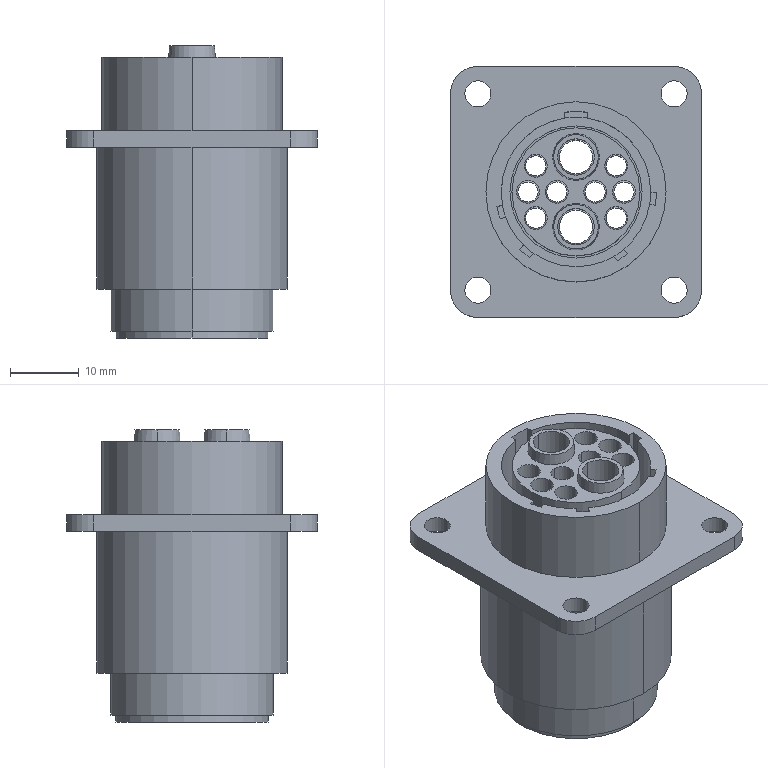Part | STEP file | 51D1-5.stp.STEP | 1 solid | 178 faces | box 36.45 x 36.45 x 42.418 mm | volume 17757 mm3 | cylinder 104 | cone 40 | plane 34 | commonest cylinder face diameters 3.326 x16 3.327 x16 21.718 x11 2.918 x8 2.921 x8 3.8 x8